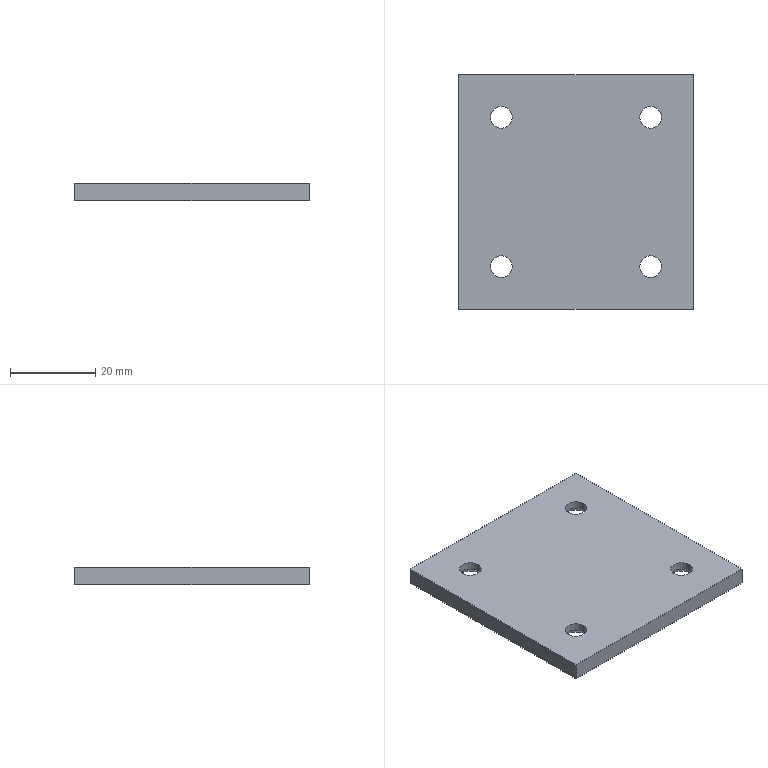Part | SolidWorks | features Chamfer 1, Extrusion 1, HoleWzd 1 | 1 solid | 22 faces | box 55 x 55 x 4 mm | volume 11573 mm3 | cone 8 | cylinder 8 | plane 6 | commonest cylinder face diameters 5.1 x8
STEP:
#1=CARTESIAN_POINT('',(20.05,17.5,2.2));
#2=VERTEX_POINT('',#1);
#3=CARTESIAN_POINT('',(14.95,17.5,2.2));
#4=VERTEX_POINT('',#3);
#5=CARTESIAN_POINT('',(17.5,17.5,2.2));
#6=DIRECTION('',(0.,0.,-1.));
#7=DIRECTION('',(1.,0.,0.));
#8=AXIS2_PLACEMENT_3D('',#5,#6,#7);
#9=CIRCLE('',#8,2.55);
#10=EDGE_CURVE('',#2,#4,#9,.T.);
#11=ORIENTED_EDGE('',*,*,#10,.F.);
#12=CARTESIAN_POINT('',(22.25,17.5,0.));
#13=VERTEX_POINT('',#12);
#14=CARTESIAN_POINT('',(20.05,17.5,2.2));
#15=DIRECTION('',(0.7071,0.,-0.7071));
#16=VECTOR('',#15,1000.);
#17=LINE('',#14,#16);
#18=EDGE_CURVE('',#2,#13,#17,.T.);
#19=ORIENTED_EDGE('',*,*,#18,.T.);
#20=CARTESIAN_POINT('',(12.75,17.5,0.));
#21=VERTEX_POINT('',#20);
#22=CARTESIAN_POINT('',(17.5,17.5,0.));
#23=DIRECTION('',(0.,0.,1.));
#24=DIRECTION('',(1.,0.,0.));
#25=AXIS2_PLACEMENT_3D('',#22,#23,#24);
#26=CIRCLE('',#25,4.75);
#27=EDGE_CURVE('',#21,#13,#26,.T.);
#28=ORIENTED_EDGE('',*,*,#27,.F.);
#29=CARTESIAN_POINT('',(14.95,17.5,2.2));
#30=DIRECTION('',(-0.7071,0.,-0.7071));
#31=VECTOR('',#30,1000.);
#32=LINE('',#29,#31);
#33=EDGE_CURVE('',#4,#21,#32,.T.);
#34=ORIENTED_EDGE('',*,*,#33,.F.);
#35=EDGE_LOOP('',(#11,#19,#28,#34));
#36=FACE_OUTER_BOUND('',#35,.T.);
#37=CARTESIAN_POINT('',(17.5,17.5,2.2));
#38=DIRECTION('',(0.,0.,-1.));
#39=DIRECTION('',(-1.,0.,0.));
#40=AXIS2_PLACEMENT_3D('',#37,#38,#39);
#41=CONICAL_SURFACE('',#40,2.55,0.7854);
#42=ADVANCED_FACE('',(#36),#41,.F.);
#43=CARTESIAN_POINT('',(-14.95,17.5,2.2));
#44=VERTEX_POINT('',#43);
#45=CARTESIAN_POINT('',(-20.05,17.5,2.2));
#46=VERTEX_POINT('',#45);
#47=CARTESIAN_POINT('',(-17.5,17.5,2.2));
#48=DIRECTION('',(0.,0.,-1.));
#49=DIRECTION('',(1.,0.,0.));
#50=AXIS2_PLACEMENT_3D('',#47,#48,#49);
#51=CIRCLE('',#50,2.55);
#52=EDGE_CURVE('',#44,#46,#51,.T.);
#53=ORIENTED_EDGE('',*,*,#52,.F.);
#54=CARTESIAN_POINT('',(-12.75,17.5,0.));
#55=VERTEX_POINT('',#54);
#56=CARTESIAN_POINT('',(-14.95,17.5,2.2));
#57=DIRECTION('',(0.7071,0.,-0.7071));
#58=VECTOR('',#57,1000.);
#59=LINE('',#56,#58);
#60=EDGE_CURVE('',#44,#55,#59,.T.);
#61=ORIENTED_EDGE('',*,*,#60,.T.);
#62=CARTESIAN_POINT('',(-22.25,17.5,0.));
#63=VERTEX_POINT('',#62);
#64=CARTESIAN_POINT('',(-17.5,17.5,0.));
#65=DIRECTION('',(0.,0.,1.));
#66=DIRECTION('',(1.,0.,0.));
#67=AXIS2_PLACEMENT_3D('',#64,#65,#66);
#68=CIRCLE('',#67,4.75);
#69=EDGE_CURVE('',#63,#55,#68,.T.);
#70=ORIENTED_EDGE('',*,*,#69,.F.);
#71=CARTESIAN_POINT('',(-20.05,17.5,2.2));
#72=DIRECTION('',(-0.7071,0.,-0.7071));
#73=VECTOR('',#72,1000.);
#74=LINE('',#71,#73);
#75=EDGE_CURVE('',#46,#63,#74,.T.);
#76=ORIENTED_EDGE('',*,*,#75,.F.);
#77=EDGE_LOOP('',(#53,#61,#70,#76));
#78=FACE_OUTER_BOUND('',#77,.T.);
#79=CARTESIAN_POINT('',(-17.5,17.5,2.2));
#80=DIRECTION('',(0.,0.,-1.));
#81=DIRECTION('',(-1.,0.,0.));
#82=AXIS2_PLACEMENT_3D('',#79,#80,#81);
#83=CONICAL_SURFACE('',#82,2.55,0.7854);
#84=ADVANCED_FACE('',(#78),#83,.F.);
#85=CARTESIAN_POINT('',(-14.95,-17.5,2.2));
#86=VERTEX_POINT('',#85);
#87=CARTESIAN_POINT('',(-20.05,-17.5,2.2));
#88=VERTEX_POINT('',#87);
#89=CARTESIAN_POINT('',(-17.5,-17.5,2.2));
#90=DIRECTION('',(0.,0.,-1.));
#91=DIRECTION('',(1.,0.,0.));
#92=AXIS2_PLACEMENT_3D('',#89,#90,#91);
#93=CIRCLE('',#92,2.55);
#94=EDGE_CURVE('',#86,#88,#93,.T.);
#95=ORIENTED_EDGE('',*,*,#94,.F.);
#96=CARTESIAN_POINT('',(-12.75,-17.5,0.));
#97=VERTEX_POINT('',#96);
#98=CARTESIAN_POINT('',(-14.95,-17.5,2.2));
#99=DIRECTION('',(0.7071,0.,-0.7071));
#100=VECTOR('',#99,1000.);
#101=LINE('',#98,#100);
#102=EDGE_CURVE('',#86,#97,#101,.T.);
#103=ORIENTED_EDGE('',*,*,#102,.T.);
#104=CARTESIAN_POINT('',(-22.25,-17.5,0.));
#105=VERTEX_POINT('',#104);
#106=CARTESIAN_POINT('',(-17.5,-17.5,0.));
#107=DIRECTION('',(0.,0.,1.));
#108=DIRECTION('',(1.,0.,0.));
#109=AXIS2_PLACEMENT_3D('',#106,#107,#108);
#110=CIRCLE('',#109,4.75);
#111=EDGE_CURVE('',#105,#97,#110,.T.);
#112=ORIENTED_EDGE('',*,*,#111,.F.);
#113=CARTESIAN_POINT('',(-20.05,-17.5,2.2));
#114=DIRECTION('',(-0.7071,0.,-0.7071));
#115=VECTOR('',#114,1000.);
#116=LINE('',#113,#115);
#117=EDGE_CURVE('',#88,#105,#116,.T.);
#118=ORIENTED_EDGE('',*,*,#117,.F.);
#119=EDGE_LOOP('',(#95,#103,#112,#118));
#120=FACE_OUTER_BOUND('',#119,.T.);
#121=CARTESIAN_POINT('',(-17.5,-17.5,2.2));
#122=DIRECTION('',(0.,0.,-1.));
#123=DIRECTION('',(-1.,0.,0.));
#124=AXIS2_PLACEMENT_3D('',#121,#122,#123);
#125=CONICAL_SURFACE('',#124,2.55,0.7854);
#126=ADVANCED_FACE('',(#120),#125,.F.);
#127=CARTESIAN_POINT('',(20.05,-17.5,2.2));
#128=VERTEX_POINT('',#127);
#129=CARTESIAN_POINT('',(14.95,-17.5,2.2));
#130=VERTEX_POINT('',#129);
#131=CARTESIAN_POINT('',(17.5,-17.5,2.2));
#132=DIRECTION('',(0.,0.,-1.));
#133=DIRECTION('',(1.,0.,0.));
#134=AXIS2_PLACEMENT_3D('',#131,#132,#133);
#135=CIRCLE('',#134,2.55);
#136=EDGE_CURVE('',#128,#130,#135,.T.);
#137=ORIENTED_EDGE('',*,*,#136,.F.);
#138=CARTESIAN_POINT('',(22.25,-17.5,0.));
#139=VERTEX_POINT('',#138);
#140=CARTESIAN_POINT('',(20.05,-17.5,2.2));
#141=DIRECTION('',(0.7071,0.,-0.7071));
#142=VECTOR('',#141,1000.);
#143=LINE('',#140,#142);
#144=EDGE_CURVE('',#128,#139,#143,.T.);
#145=ORIENTED_EDGE('',*,*,#144,.T.);
#146=CARTESIAN_POINT('',(12.75,-17.5,0.));
#147=VERTEX_POINT('',#146);
#148=CARTESIAN_POINT('',(17.5,-17.5,0.));
#149=DIRECTION('',(0.,0.,1.));
#150=DIRECTION('',(1.,0.,0.));
#151=AXIS2_PLACEMENT_3D('',#148,#149,#150);
#152=CIRCLE('',#151,4.75);
#153=EDGE_CURVE('',#147,#139,#152,.T.);
#154=ORIENTED_EDGE('',*,*,#153,.F.);
#155=CARTESIAN_POINT('',(14.95,-17.5,2.2));
#156=DIRECTION('',(-0.7071,0.,-0.7071));
#157=VECTOR('',#156,1000.);
#158=LINE('',#155,#157);
#159=EDGE_CURVE('',#130,#147,#158,.T.);
#160=ORIENTED_EDGE('',*,*,#159,.F.);
#161=EDGE_LOOP('',(#137,#145,#154,#160));
#162=FACE_OUTER_BOUND('',#161,.T.);
#163=CARTESIAN_POINT('',(17.5,-17.5,2.2));
#164=DIRECTION('',(0.,0.,-1.));
#165=DIRECTION('',(-1.,0.,0.));
#166=AXIS2_PLACEMENT_3D('',#163,#164,#165);
#167=CONICAL_SURFACE('',#166,2.55,0.7854);
#168=ADVANCED_FACE('',(#162),#167,.F.);
#169=CARTESIAN_POINT('',(20.05,17.5,4.));
#170=VERTEX_POINT('',#169);
#171=CARTESIAN_POINT('',(14.95,17.5,4.));
#172=VERTEX_POINT('',#171);
#173=CARTESIAN_POINT('',(17.5,17.5,4.));
#174=DIRECTION('',(0.,0.,-1.));
#175=DIRECTION('',(-1.,0.,0.));
#176=AXIS2_PLACEMENT_3D('',#173,#174,#175);
#177=CIRCLE('',#176,2.55);
#178=EDGE_CURVE('',#170,#172,#177,.T.);
#179=ORIENTED_EDGE('',*,*,#178,.F.);
#180=CARTESIAN_POINT('',(20.05,17.5,0.));
#181=DIRECTION('',(0.,0.,-1.));
#182=VECTOR('',#181,1000.);
#183=LINE('',#180,#182);
#184=EDGE_CURVE('',#170,#2,#183,.T.);
#185=ORIENTED_EDGE('',*,*,#184,.T.);
#186=ORIENTED_EDGE('',*,*,#10,.T.);
#187=CARTESIAN_POINT('',(14.95,17.5,0.));
#188=DIRECTION('',(0.,0.,-1.));
#189=VECTOR('',#188,1000.);
#190=LINE('',#187,#189);
#191=EDGE_CURVE('',#172,#4,#190,.T.);
#192=ORIENTED_EDGE('',*,*,#191,.F.);
#193=EDGE_LOOP('',(#179,#185,#186,#192));
#194=FACE_OUTER_BOUND('',#193,.T.);
#195=CARTESIAN_POINT('',(17.5,17.5,0.));
#196=DIRECTION('',(0.,0.,-1.));
#197=DIRECTION('',(-1.,0.,0.));
#198=AXIS2_PLACEMENT_3D('',#195,#196,#197);
#199=CYLINDRICAL_SURFACE('',#198,2.55);
#200=ADVANCED_FACE('',(#194),#199,.F.);
#201=CARTESIAN_POINT('',(-14.95,17.5,4.));
#202=VERTEX_POINT('',#201);
#203=CARTESIAN_POINT('',(-20.05,17.5,4.));
#204=VERTEX_POINT('',#203);
#205=CARTESIAN_POINT('',(-17.5,17.5,4.));
#206=DIRECTION('',(0.,0.,-1.));
#207=DIRECTION('',(-1.,0.,0.));
#208=AXIS2_PLACEMENT_3D('',#205,#206,#207);
#209=CIRCLE('',#208,2.55);
#210=EDGE_CURVE('',#202,#204,#209,.T.);
#211=ORIENTED_EDGE('',*,*,#210,.F.);
#212=CARTESIAN_POINT('',(-14.95,17.5,0.));
#213=DIRECTION('',(0.,0.,-1.));
#214=VECTOR('',#213,1000.);
#215=LINE('',#212,#214);
#216=EDGE_CURVE('',#202,#44,#215,.T.);
#217=ORIENTED_EDGE('',*,*,#216,.T.);
#218=ORIENTED_EDGE('',*,*,#52,.T.);
#219=CARTESIAN_POINT('',(-20.05,17.5,0.));
#220=DIRECTION('',(0.,0.,-1.));
#221=VECTOR('',#220,1000.);
#222=LINE('',#219,#221);
#223=EDGE_CURVE('',#204,#46,#222,.T.);
#224=ORIENTED_EDGE('',*,*,#223,.F.);
#225=EDGE_LOOP('',(#211,#217,#218,#224));
#226=FACE_OUTER_BOUND('',#225,.T.);
#227=CARTESIAN_POINT('',(-17.5,17.5,0.));
#228=DIRECTION('',(0.,0.,-1.));
#229=DIRECTION('',(-1.,0.,0.));
#230=AXIS2_PLACEMENT_3D('',#227,#228,#229);
#231=CYLINDRICAL_SURFACE('',#230,2.55);
#232=ADVANCED_FACE('',(#226),#231,.F.);
#233=CARTESIAN_POINT('',(-14.95,-17.5,4.));
#234=VERTEX_POINT('',#233);
#235=CARTESIAN_POINT('',(-20.05,-17.5,4.));
#236=VERTEX_POINT('',#235);
#237=CARTESIAN_POINT('',(-17.5,-17.5,4.));
#238=DIRECTION('',(0.,0.,-1.));
#239=DIRECTION('',(-1.,0.,0.));
#240=AXIS2_PLACEMENT_3D('',#237,#238,#239);
#241=CIRCLE('',#240,2.55);
#242=EDGE_CURVE('',#234,#236,#241,.T.);
#243=ORIENTED_EDGE('',*,*,#242,.F.);
#244=CARTESIAN_POINT('',(-14.95,-17.5,0.));
#245=DIRECTION('',(0.,0.,-1.));
#246=VECTOR('',#245,1000.);
#247=LINE('',#244,#246);
#248=EDGE_CURVE('',#234,#86,#247,.T.);
#249=ORIENTED_EDGE('',*,*,#248,.T.);
#250=ORIENTED_EDGE('',*,*,#94,.T.);
#251=CARTESIAN_POINT('',(-20.05,-17.5,0.));
#252=DIRECTION('',(0.,0.,-1.));
#253=VECTOR('',#252,1000.);
#254=LINE('',#251,#253);
#255=EDGE_CURVE('',#236,#88,#254,.T.);
#256=ORIENTED_EDGE('',*,*,#255,.F.);
#257=EDGE_LOOP('',(#243,#249,#250,#256));
#258=FACE_OUTER_BOUND('',#257,.T.);
#259=CARTESIAN_POINT('',(-17.5,-17.5,0.));
#260=DIRECTION('',(0.,0.,-1.));
#261=DIRECTION('',(-1.,0.,0.));
#262=AXIS2_PLACEMENT_3D('',#259,#260,#261);
#263=CYLINDRICAL_SURFACE('',#262,2.55);
#264=ADVANCED_FACE('',(#258),#263,.F.);
#265=CARTESIAN_POINT('',(20.05,-17.5,4.));
#266=VERTEX_POINT('',#265);
#267=CARTESIAN_POINT('',(14.95,-17.5,4.));
#268=VERTEX_POINT('',#267);
#269=CARTESIAN_POINT('',(17.5,-17.5,4.));
#270=DIRECTION('',(0.,0.,-1.));
#271=DIRECTION('',(-1.,0.,0.));
#272=AXIS2_PLACEMENT_3D('',#269,#270,#271);
#273=CIRCLE('',#272,2.55);
#274=EDGE_CURVE('',#266,#268,#273,.T.);
#275=ORIENTED_EDGE('',*,*,#274,.F.);
#276=CARTESIAN_POINT('',(20.05,-17.5,0.));
#277=DIRECTION('',(0.,0.,-1.));
#278=VECTOR('',#277,1000.);
#279=LINE('',#276,#278);
#280=EDGE_CURVE('',#266,#128,#279,.T.);
#281=ORIENTED_EDGE('',*,*,#280,.T.);
#282=ORIENTED_EDGE('',*,*,#136,.T.);
#283=CARTESIAN_POINT('',(14.95,-17.5,0.));
#284=DIRECTION('',(0.,0.,-1.));
#285=VECTOR('',#284,1000.);
#286=LINE('',#283,#285);
#287=EDGE_CURVE('',#268,#130,#286,.T.);
#288=ORIENTED_EDGE('',*,*,#287,.F.);
#289=EDGE_LOOP('',(#275,#281,#282,#288));
#290=FACE_OUTER_BOUND('',#289,.T.);
#291=CARTESIAN_POINT('',(17.5,-17.5,0.));
#292=DIRECTION('',(0.,0.,-1.));
#293=DIRECTION('',(-1.,0.,0.));
#294=AXIS2_PLACEMENT_3D('',#291,#292,#293);
#295=CYLINDRICAL_SURFACE('',#294,2.55);
#296=ADVANCED_FACE('',(#290),#295,.F.);
#297=CARTESIAN_POINT('',(-27.5,-27.5,4.));
#298=VERTEX_POINT('',#297);
#299=CARTESIAN_POINT('',(27.5,-27.5,4.));
#300=VERTEX_POINT('',#299);
#301=CARTESIAN_POINT('',(0.,-27.5,4.));
#302=DIRECTION('',(1.,0.,0.));
#303=VECTOR('',#302,1000.);
#304=LINE('',#301,#303);
#305=EDGE_CURVE('',#298,#300,#304,.T.);
#306=ORIENTED_EDGE('',*,*,#305,.T.);
#307=CARTESIAN_POINT('',(27.5,27.5,4.));
#308=VERTEX_POINT('',#307);
#309=CARTESIAN_POINT('',(27.5,0.,4.));
#310=DIRECTION('',(0.,1.,0.));
#311=VECTOR('',#310,1000.);
#312=LINE('',#309,#311);
#313=EDGE_CURVE('',#300,#308,#312,.T.);
#314=ORIENTED_EDGE('',*,*,#313,.T.);
#315=CARTESIAN_POINT('',(-27.5,27.5,4.));
#316=VERTEX_POINT('',#315);
#317=CARTESIAN_POINT('',(0.,27.5,4.));
#318=DIRECTION('',(1.,0.,0.));
#319=VECTOR('',#318,1000.);
#320=LINE('',#317,#319);
#321=EDGE_CURVE('',#316,#308,#320,.T.);
#322=ORIENTED_EDGE('',*,*,#321,.F.);
#323=CARTESIAN_POINT('',(-27.5,0.,4.));
#324=DIRECTION('',(0.,1.,0.));
#325=VECTOR('',#324,1000.);
#326=LINE('',#323,#325);
#327=EDGE_CURVE('',#298,#316,#326,.T.);
#328=ORIENTED_EDGE('',*,*,#327,.F.);
#329=EDGE_LOOP('',(#306,#314,#322,#328));
#330=FACE_OUTER_BOUND('',#329,.T.);
#331=CARTESIAN_POINT('',(17.5,-17.5,4.));
#332=DIRECTION('',(0.,0.,-1.));
#333=DIRECTION('',(-1.,0.,0.));
#334=AXIS2_PLACEMENT_3D('',#331,#332,#333);
#335=CIRCLE('',#334,2.55);
#336=EDGE_CURVE('',#268,#266,#335,.T.);
#337=ORIENTED_EDGE('',*,*,#336,.T.);
#338=ORIENTED_EDGE('',*,*,#274,.T.);
#339=EDGE_LOOP('',(#337,#338));
#340=FACE_BOUND('',#339,.T.);
#341=CARTESIAN_POINT('',(-17.5,-17.5,4.));
#342=DIRECTION('',(0.,0.,-1.));
#343=DIRECTION('',(-1.,0.,0.));
#344=AXIS2_PLACEMENT_3D('',#341,#342,#343);
#345=CIRCLE('',#344,2.55);
#346=EDGE_CURVE('',#236,#234,#345,.T.);
#347=ORIENTED_EDGE('',*,*,#346,.T.);
#348=ORIENTED_EDGE('',*,*,#242,.T.);
#349=EDGE_LOOP('',(#347,#348));
#350=FACE_BOUND('',#349,.T.);
#351=CARTESIAN_POINT('',(-17.5,17.5,4.));
#352=DIRECTION('',(0.,0.,-1.));
#353=DIRECTION('',(-1.,0.,0.));
#354=AXIS2_PLACEMENT_3D('',#351,#352,#353);
#355=CIRCLE('',#354,2.55);
#356=EDGE_CURVE('',#204,#202,#355,.T.);
#357=ORIENTED_EDGE('',*,*,#356,.T.);
#358=ORIENTED_EDGE('',*,*,#210,.T.);
#359=EDGE_LOOP('',(#357,#358));
#360=FACE_BOUND('',#359,.T.);
#361=CARTESIAN_POINT('',(17.5,17.5,4.));
#362=DIRECTION('',(0.,0.,-1.));
#363=DIRECTION('',(-1.,0.,0.));
#364=AXIS2_PLACEMENT_3D('',#361,#362,#363);
#365=CIRCLE('',#364,2.55);
#366=EDGE_CURVE('',#172,#170,#365,.T.);
#367=ORIENTED_EDGE('',*,*,#366,.T.);
#368=ORIENTED_EDGE('',*,*,#178,.T.);
#369=EDGE_LOOP('',(#367,#368));
#370=FACE_BOUND('',#369,.T.);
#371=CARTESIAN_POINT('',(0.,0.,4.));
#372=DIRECTION('',(0.,0.,1.));
#373=DIRECTION('',(1.,0.,0.));
#374=AXIS2_PLACEMENT_3D('',#371,#372,#373);
#375=PLANE('',#374);
#376=ADVANCED_FACE('',(#330,#340,#350,#360,#370),#375,.T.);
#377=ORIENTED_EDGE('',*,*,#153,.T.);
#378=CARTESIAN_POINT('',(17.5,-17.5,0.));
#379=DIRECTION('',(0.,0.,1.));
#380=DIRECTION('',(1.,0.,0.));
#381=AXIS2_PLACEMENT_3D('',#378,#379,#380);
#382=CIRCLE('',#381,4.75);
#383=EDGE_CURVE('',#139,#147,#382,.T.);
#384=ORIENTED_EDGE('',*,*,#383,.T.);
#385=EDGE_LOOP('',(#377,#384));
#386=FACE_BOUND('',#385,.T.);
#387=ORIENTED_EDGE('',*,*,#111,.T.);
#388=CARTESIAN_POINT('',(-17.5,-17.5,0.));
#389=DIRECTION('',(0.,0.,1.));
#390=DIRECTION('',(1.,0.,0.));
#391=AXIS2_PLACEMENT_3D('',#388,#389,#390);
#392=CIRCLE('',#391,4.75);
#393=EDGE_CURVE('',#97,#105,#392,.T.);
#394=ORIENTED_EDGE('',*,*,#393,.T.);
#395=EDGE_LOOP('',(#387,#394));
#396=FACE_BOUND('',#395,.T.);
#397=ORIENTED_EDGE('',*,*,#69,.T.);
#398=CARTESIAN_POINT('',(-17.5,17.5,0.));
#399=DIRECTION('',(0.,0.,1.));
#400=DIRECTION('',(1.,0.,0.));
#401=AXIS2_PLACEMENT_3D('',#398,#399,#400);
#402=CIRCLE('',#401,4.75);
#403=EDGE_CURVE('',#55,#63,#402,.T.);
#404=ORIENTED_EDGE('',*,*,#403,.T.);
#405=EDGE_LOOP('',(#397,#404));
#406=FACE_BOUND('',#405,.T.);
#407=ORIENTED_EDGE('',*,*,#27,.T.);
#408=CARTESIAN_POINT('',(17.5,17.5,0.));
#409=DIRECTION('',(0.,0.,1.));
#410=DIRECTION('',(1.,0.,0.));
#411=AXIS2_PLACEMENT_3D('',#408,#409,#410);
#412=CIRCLE('',#411,4.75);
#413=EDGE_CURVE('',#13,#21,#412,.T.);
#414=ORIENTED_EDGE('',*,*,#413,.T.);
#415=EDGE_LOOP('',(#407,#414));
#416=FACE_BOUND('',#415,.T.);
#417=CARTESIAN_POINT('',(-27.5,-27.5,0.));
#418=VERTEX_POINT('',#417);
#419=CARTESIAN_POINT('',(27.5,-27.5,0.));
#420=VERTEX_POINT('',#419);
#421=CARTESIAN_POINT('',(0.,-27.5,0.));
#422=DIRECTION('',(1.,0.,0.));
#423=VECTOR('',#422,1000.);
#424=LINE('',#421,#423);
#425=EDGE_CURVE('',#418,#420,#424,.T.);
#426=ORIENTED_EDGE('',*,*,#425,.F.);
#427=CARTESIAN_POINT('',(-27.5,27.5,0.));
#428=VERTEX_POINT('',#427);
#429=CARTESIAN_POINT('',(-27.5,0.,0.));
#430=DIRECTION('',(0.,1.,0.));
#431=VECTOR('',#430,1000.);
#432=LINE('',#429,#431);
#433=EDGE_CURVE('',#418,#428,#432,.T.);
#434=ORIENTED_EDGE('',*,*,#433,.T.);
#435=CARTESIAN_POINT('',(27.5,27.5,0.));
#436=VERTEX_POINT('',#435);
#437=CARTESIAN_POINT('',(0.,27.5,0.));
#438=DIRECTION('',(1.,0.,0.));
#439=VECTOR('',#438,1000.);
#440=LINE('',#437,#439);
#441=EDGE_CURVE('',#428,#436,#440,.T.);
#442=ORIENTED_EDGE('',*,*,#441,.T.);
#443=CARTESIAN_POINT('',(27.5,0.,0.));
#444=DIRECTION('',(0.,1.,0.));
#445=VECTOR('',#444,1000.);
#446=LINE('',#443,#445);
#447=EDGE_CURVE('',#420,#436,#446,.T.);
#448=ORIENTED_EDGE('',*,*,#447,.F.);
#449=EDGE_LOOP('',(#426,#434,#442,#448));
#450=FACE_OUTER_BOUND('',#449,.T.);
#451=CARTESIAN_POINT('',(0.,0.,0.));
#452=DIRECTION('',(0.,0.,1.));
#453=DIRECTION('',(1.,0.,0.));
#454=AXIS2_PLACEMENT_3D('',#451,#452,#453);
#455=PLANE('',#454);
#456=ADVANCED_FACE('',(#386,#396,#406,#416,#450),#455,.F.);
#457=ORIENTED_EDGE('',*,*,#447,.T.);
#458=CARTESIAN_POINT('',(27.5,27.5,4.));
#459=DIRECTION('',(0.,0.,-1.));
#460=VECTOR('',#459,1000.);
#461=LINE('',#458,#460);
#462=EDGE_CURVE('',#308,#436,#461,.T.);
#463=ORIENTED_EDGE('',*,*,#462,.F.);
#464=ORIENTED_EDGE('',*,*,#313,.F.);
#465=CARTESIAN_POINT('',(27.5,-27.5,4.));
#466=DIRECTION('',(0.,0.,-1.));
#467=VECTOR('',#466,1000.);
#468=LINE('',#465,#467);
#469=EDGE_CURVE('',#300,#420,#468,.T.);
#470=ORIENTED_EDGE('',*,*,#469,.T.);
#471=EDGE_LOOP('',(#457,#463,#464,#470));
#472=FACE_OUTER_BOUND('',#471,.T.);
#473=CARTESIAN_POINT('',(27.5,0.,4.));
#474=DIRECTION('',(-1.,0.,0.));
#475=DIRECTION('',(0.,0.,1.));
#476=AXIS2_PLACEMENT_3D('',#473,#474,#475);
#477=PLANE('',#476);
#478=ADVANCED_FACE('',(#472),#477,.F.);
#479=ORIENTED_EDGE('',*,*,#441,.F.);
#480=CARTESIAN_POINT('',(-27.5,27.5,4.));
#481=DIRECTION('',(0.,0.,-1.));
#482=VECTOR('',#481,1000.);
#483=LINE('',#480,#482);
#484=EDGE_CURVE('',#316,#428,#483,.T.);
#485=ORIENTED_EDGE('',*,*,#484,.F.);
#486=ORIENTED_EDGE('',*,*,#321,.T.);
#487=ORIENTED_EDGE('',*,*,#462,.T.);
#488=EDGE_LOOP('',(#479,#485,#486,#487));
#489=FACE_OUTER_BOUND('',#488,.T.);
#490=CARTESIAN_POINT('',(0.,27.5,4.));
#491=DIRECTION('',(0.,1.,0.));
#492=DIRECTION('',(0.,0.,1.));
#493=AXIS2_PLACEMENT_3D('',#490,#491,#492);
#494=PLANE('',#493);
#495=ADVANCED_FACE('',(#489),#494,.T.);
#496=ORIENTED_EDGE('',*,*,#433,.F.);
#497=CARTESIAN_POINT('',(-27.5,-27.5,4.));
#498=DIRECTION('',(0.,0.,-1.));
#499=VECTOR('',#498,1000.);
#500=LINE('',#497,#499);
#501=EDGE_CURVE('',#298,#418,#500,.T.);
#502=ORIENTED_EDGE('',*,*,#501,.F.);
#503=ORIENTED_EDGE('',*,*,#327,.T.);
#504=ORIENTED_EDGE('',*,*,#484,.T.);
#505=EDGE_LOOP('',(#496,#502,#503,#504));
#506=FACE_OUTER_BOUND('',#505,.T.);
#507=CARTESIAN_POINT('',(-27.5,0.,4.));
#508=DIRECTION('',(-1.,0.,0.));
#509=DIRECTION('',(0.,0.,1.));
#510=AXIS2_PLACEMENT_3D('',#507,#508,#509);
#511=PLANE('',#510);
#512=ADVANCED_FACE('',(#506),#511,.T.);
#513=ORIENTED_EDGE('',*,*,#425,.T.);
#514=ORIENTED_EDGE('',*,*,#469,.F.);
#515=ORIENTED_EDGE('',*,*,#305,.F.);
#516=ORIENTED_EDGE('',*,*,#501,.T.);
#517=EDGE_LOOP('',(#513,#514,#515,#516));
#518=FACE_OUTER_BOUND('',#517,.T.);
#519=CARTESIAN_POINT('',(0.,-27.5,4.));
#520=DIRECTION('',(0.,1.,0.));
#521=DIRECTION('',(0.,0.,1.));
#522=AXIS2_PLACEMENT_3D('',#519,#520,#521);
#523=PLANE('',#522);
#524=ADVANCED_FACE('',(#518),#523,.F.);
#525=ORIENTED_EDGE('',*,*,#280,.F.);
#526=ORIENTED_EDGE('',*,*,#336,.F.);
#527=ORIENTED_EDGE('',*,*,#287,.T.);
#528=CARTESIAN_POINT('',(17.5,-17.5,2.2));
#529=DIRECTION('',(0.,0.,-1.));
#530=DIRECTION('',(1.,0.,0.));
#531=AXIS2_PLACEMENT_3D('',#528,#529,#530);
#532=CIRCLE('',#531,2.55);
#533=EDGE_CURVE('',#130,#128,#532,.T.);
#534=ORIENTED_EDGE('',*,*,#533,.T.);
#535=EDGE_LOOP('',(#525,#526,#527,#534));
#536=FACE_OUTER_BOUND('',#535,.T.);
#537=CARTESIAN_POINT('',(17.5,-17.5,0.));
#538=DIRECTION('',(0.,0.,-1.));
#539=DIRECTION('',(-1.,0.,0.));
#540=AXIS2_PLACEMENT_3D('',#537,#538,#539);
#541=CYLINDRICAL_SURFACE('',#540,2.55);
#542=ADVANCED_FACE('',(#536),#541,.F.);
#543=ORIENTED_EDGE('',*,*,#248,.F.);
#544=ORIENTED_EDGE('',*,*,#346,.F.);
#545=ORIENTED_EDGE('',*,*,#255,.T.);
#546=CARTESIAN_POINT('',(-17.5,-17.5,2.2));
#547=DIRECTION('',(0.,0.,-1.));
#548=DIRECTION('',(1.,0.,0.));
#549=AXIS2_PLACEMENT_3D('',#546,#547,#548);
#550=CIRCLE('',#549,2.55);
#551=EDGE_CURVE('',#88,#86,#550,.T.);
#552=ORIENTED_EDGE('',*,*,#551,.T.);
#553=EDGE_LOOP('',(#543,#544,#545,#552));
#554=FACE_OUTER_BOUND('',#553,.T.);
#555=CARTESIAN_POINT('',(-17.5,-17.5,0.));
#556=DIRECTION('',(0.,0.,-1.));
#557=DIRECTION('',(-1.,0.,0.));
#558=AXIS2_PLACEMENT_3D('',#555,#556,#557);
#559=CYLINDRICAL_SURFACE('',#558,2.55);
#560=ADVANCED_FACE('',(#554),#559,.F.);
#561=ORIENTED_EDGE('',*,*,#216,.F.);
#562=ORIENTED_EDGE('',*,*,#356,.F.);
#563=ORIENTED_EDGE('',*,*,#223,.T.);
#564=CARTESIAN_POINT('',(-17.5,17.5,2.2));
#565=DIRECTION('',(0.,0.,-1.));
#566=DIRECTION('',(1.,0.,0.));
#567=AXIS2_PLACEMENT_3D('',#564,#565,#566);
#568=CIRCLE('',#567,2.55);
#569=EDGE_CURVE('',#46,#44,#568,.T.);
#570=ORIENTED_EDGE('',*,*,#569,.T.);
#571=EDGE_LOOP('',(#561,#562,#563,#570));
#572=FACE_OUTER_BOUND('',#571,.T.);
#573=CARTESIAN_POINT('',(-17.5,17.5,0.));
#574=DIRECTION('',(0.,0.,-1.));
#575=DIRECTION('',(-1.,0.,0.));
#576=AXIS2_PLACEMENT_3D('',#573,#574,#575);
#577=CYLINDRICAL_SURFACE('',#576,2.55);
#578=ADVANCED_FACE('',(#572),#577,.F.);
#579=ORIENTED_EDGE('',*,*,#184,.F.);
#580=ORIENTED_EDGE('',*,*,#366,.F.);
#581=ORIENTED_EDGE('',*,*,#191,.T.);
#582=CARTESIAN_POINT('',(17.5,17.5,2.2));
#583=DIRECTION('',(0.,0.,-1.));
#584=DIRECTION('',(1.,0.,0.));
#585=AXIS2_PLACEMENT_3D('',#582,#583,#584);
#586=CIRCLE('',#585,2.55);
#587=EDGE_CURVE('',#4,#2,#586,.T.);
#588=ORIENTED_EDGE('',*,*,#587,.T.);
#589=EDGE_LOOP('',(#579,#580,#581,#588));
#590=FACE_OUTER_BOUND('',#589,.T.);
#591=CARTESIAN_POINT('',(17.5,17.5,0.));
#592=DIRECTION('',(0.,0.,-1.));
#593=DIRECTION('',(-1.,0.,0.));
#594=AXIS2_PLACEMENT_3D('',#591,#592,#593);
#595=CYLINDRICAL_SURFACE('',#594,2.55);
#596=ADVANCED_FACE('',(#590),#595,.F.);
#597=ORIENTED_EDGE('',*,*,#144,.F.);
#598=ORIENTED_EDGE('',*,*,#533,.F.);
#599=ORIENTED_EDGE('',*,*,#159,.T.);
#600=ORIENTED_EDGE('',*,*,#383,.F.);
#601=EDGE_LOOP('',(#597,#598,#599,#600));
#602=FACE_OUTER_BOUND('',#601,.T.);
#603=CARTESIAN_POINT('',(17.5,-17.5,2.2));
#604=DIRECTION('',(0.,0.,-1.));
#605=DIRECTION('',(-1.,0.,0.));
#606=AXIS2_PLACEMENT_3D('',#603,#604,#605);
#607=CONICAL_SURFACE('',#606,2.55,0.7854);
#608=ADVANCED_FACE('',(#602),#607,.F.);
#609=ORIENTED_EDGE('',*,*,#102,.F.);
#610=ORIENTED_EDGE('',*,*,#551,.F.);
#611=ORIENTED_EDGE('',*,*,#117,.T.);
#612=ORIENTED_EDGE('',*,*,#393,.F.);
#613=EDGE_LOOP('',(#609,#610,#611,#612));
#614=FACE_OUTER_BOUND('',#613,.T.);
#615=CARTESIAN_POINT('',(-17.5,-17.5,2.2));
#616=DIRECTION('',(0.,0.,-1.));
#617=DIRECTION('',(-1.,0.,0.));
#618=AXIS2_PLACEMENT_3D('',#615,#616,#617);
#619=CONICAL_SURFACE('',#618,2.55,0.7854);
#620=ADVANCED_FACE('',(#614),#619,.F.);
#621=ORIENTED_EDGE('',*,*,#60,.F.);
#622=ORIENTED_EDGE('',*,*,#569,.F.);
#623=ORIENTED_EDGE('',*,*,#75,.T.);
#624=ORIENTED_EDGE('',*,*,#403,.F.);
#625=EDGE_LOOP('',(#621,#622,#623,#624));
#626=FACE_OUTER_BOUND('',#625,.T.);
#627=CARTESIAN_POINT('',(-17.5,17.5,2.2));
#628=DIRECTION('',(0.,0.,-1.));
#629=DIRECTION('',(-1.,0.,0.));
#630=AXIS2_PLACEMENT_3D('',#627,#628,#629);
#631=CONICAL_SURFACE('',#630,2.55,0.7854);
#632=ADVANCED_FACE('',(#626),#631,.F.);
#633=ORIENTED_EDGE('',*,*,#18,.F.);
#634=ORIENTED_EDGE('',*,*,#587,.F.);
#635=ORIENTED_EDGE('',*,*,#33,.T.);
#636=ORIENTED_EDGE('',*,*,#413,.F.);
#637=EDGE_LOOP('',(#633,#634,#635,#636));
#638=FACE_OUTER_BOUND('',#637,.T.);
#639=CARTESIAN_POINT('',(17.5,17.5,2.2));
#640=DIRECTION('',(0.,0.,-1.));
#641=DIRECTION('',(-1.,0.,0.));
#642=AXIS2_PLACEMENT_3D('',#639,#640,#641);
#643=CONICAL_SURFACE('',#642,2.55,0.7854);
#644=ADVANCED_FACE('',(#638),#643,.F.);
#645=CLOSED_SHELL('',(#42,#84,#126,#168,#200,#232,#264,#296,#376,#456,#478,#495,#512,#524,#542,#560,#578,#596,#608,#620,#632,#644));
#646=MANIFOLD_SOLID_BREP('',#645);
#647=CARTESIAN_POINT('',(0.,0.,0.));
#648=DIRECTION('',(0.,0.,1.));
#649=DIRECTION('',(1.,0.,0.));
#650=AXIS2_PLACEMENT_3D('',#647,#648,#649);
#651=(LENGTH_UNIT()NAMED_UNIT(*)SI_UNIT(.MILLI.,.METRE.));
#652=UNCERTAINTY_MEASURE_WITH_UNIT(LENGTH_MEASURE(0.00001),#651,'','');
#653=(NAMED_UNIT(*)PLANE_ANGLE_UNIT()SI_UNIT($,.RADIAN.));
#654=(NAMED_UNIT(*)SI_UNIT($,.STERADIAN.)SOLID_ANGLE_UNIT());
#655=(GEOMETRIC_REPRESENTATION_CONTEXT(3)GLOBAL_UNCERTAINTY_ASSIGNED_CONTEXT((#652))GLOBAL_UNIT_ASSIGNED_CONTEXT((#651,#653,#654))REPRESENTATION_CONTEXT('',''));
#656=ADVANCED_BREP_SHAPE_REPRESENTATION('',(#646,#650),#655);